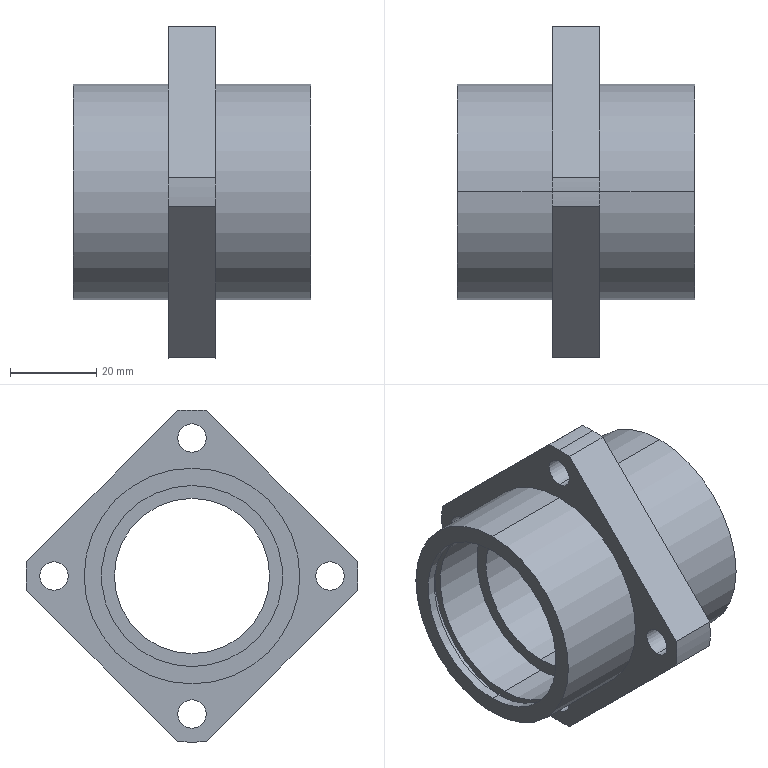Part | STEP file | _housing_bgfszb6004-55-22 | 1 solid | 57 faces | box 55 x 77 x 77 mm | volume 52579 mm3 | cylinder 39 | plane 18 | commonest cylinder face diameters 6.6 x8 11 x8 42 x8 77 x5 45.5 x4 50 x4